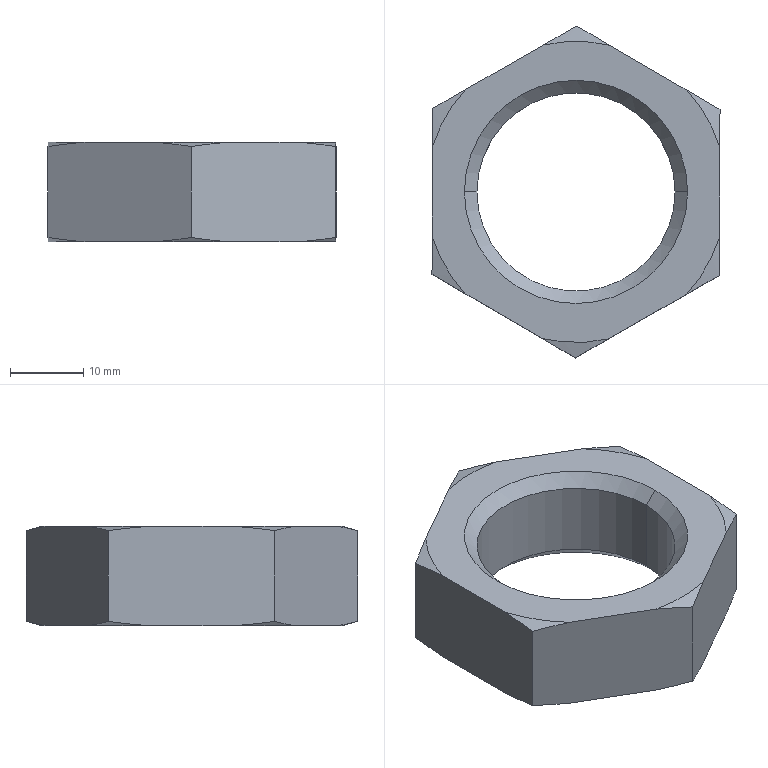Part | STEP file | GB/T6172.1-2000 hex thin nut grade A and B (M27) | 1 solid | 26 faces | box 39.233 x 45.2 x 13.5 mm | volume 9913 mm3 | cone 16 | plane 8 | cylinder 2 | commonest cylinder face diameters 27 x2
STEP:
#1=CARTESIAN_POINT('',(-13.5,0.,11.807));
#2=VERTEX_POINT('',#1);
#3=CARTESIAN_POINT('',(13.5,0.,11.807));
#4=VERTEX_POINT('',#3);
#5=CARTESIAN_POINT('',(0.,0.,11.807));
#6=DIRECTION('',(0.,0.,1.));
#7=DIRECTION('',(-1.,0.,0.));
#8=AXIS2_PLACEMENT_3D('',#5,#6,#7);
#9=CIRCLE('',#8,13.5);
#10=EDGE_CURVE('',#2,#4,#9,.T.);
#11=ORIENTED_EDGE('',*,*,#10,.F.);
#12=CARTESIAN_POINT('',(-15.193,0.,13.5));
#13=VERTEX_POINT('',#12);
#14=CARTESIAN_POINT('',(-13.5,0.,11.807));
#15=DIRECTION('',(-0.7071,0.,0.7071));
#16=VECTOR('',#15,1000.);
#17=LINE('',#14,#16);
#18=EDGE_CURVE('',#2,#13,#17,.T.);
#19=ORIENTED_EDGE('',*,*,#18,.T.);
#20=CARTESIAN_POINT('',(15.193,0.,13.5));
#21=VERTEX_POINT('',#20);
#22=CARTESIAN_POINT('',(0.,0.,13.5));
#23=DIRECTION('',(0.,0.,-1.));
#24=DIRECTION('',(-1.,0.,0.));
#25=AXIS2_PLACEMENT_3D('',#22,#23,#24);
#26=CIRCLE('',#25,15.193);
#27=EDGE_CURVE('',#21,#13,#26,.T.);
#28=ORIENTED_EDGE('',*,*,#27,.F.);
#29=CARTESIAN_POINT('',(13.5,0.,11.807));
#30=DIRECTION('',(0.7071,0.,0.7071));
#31=VECTOR('',#30,1000.);
#32=LINE('',#29,#31);
#33=EDGE_CURVE('',#4,#21,#32,.T.);
#34=ORIENTED_EDGE('',*,*,#33,.F.);
#35=EDGE_LOOP('',(#11,#19,#28,#34));
#36=FACE_OUTER_BOUND('',#35,.T.);
#37=CARTESIAN_POINT('',(0.,0.,11.807));
#38=DIRECTION('',(0.,0.,1.));
#39=DIRECTION('',(1.,0.,0.));
#40=AXIS2_PLACEMENT_3D('',#37,#38,#39);
#41=CONICAL_SURFACE('',#40,13.5,0.7854);
#42=ADVANCED_FACE('',(#36),#41,.F.);
#43=CARTESIAN_POINT('',(13.5,0.,1.693));
#44=VERTEX_POINT('',#43);
#45=CARTESIAN_POINT('',(-13.5,0.,1.693));
#46=VERTEX_POINT('',#45);
#47=CARTESIAN_POINT('',(0.,0.,1.693));
#48=DIRECTION('',(0.,0.,-1.));
#49=DIRECTION('',(-1.,0.,0.));
#50=AXIS2_PLACEMENT_3D('',#47,#48,#49);
#51=CIRCLE('',#50,13.5);
#52=EDGE_CURVE('',#44,#46,#51,.T.);
#53=ORIENTED_EDGE('',*,*,#52,.F.);
#54=CARTESIAN_POINT('',(15.193,0.,0.));
#55=VERTEX_POINT('',#54);
#56=CARTESIAN_POINT('',(15.193,0.,0.));
#57=DIRECTION('',(0.7071,0.,-0.7071));
#58=VECTOR('',#57,1000.);
#59=LINE('',#56,#58);
#60=EDGE_CURVE('',#44,#55,#59,.T.);
#61=ORIENTED_EDGE('',*,*,#60,.T.);
#62=CARTESIAN_POINT('',(-15.193,0.,0.));
#63=VERTEX_POINT('',#62);
#64=CARTESIAN_POINT('',(0.,0.,0.));
#65=DIRECTION('',(0.,0.,1.));
#66=DIRECTION('',(-1.,0.,0.));
#67=AXIS2_PLACEMENT_3D('',#64,#65,#66);
#68=CIRCLE('',#67,15.193);
#69=EDGE_CURVE('',#63,#55,#68,.T.);
#70=ORIENTED_EDGE('',*,*,#69,.F.);
#71=CARTESIAN_POINT('',(-15.193,0.,0.));
#72=DIRECTION('',(-0.7071,0.,-0.7071));
#73=VECTOR('',#72,1000.);
#74=LINE('',#71,#73);
#75=EDGE_CURVE('',#46,#63,#74,.T.);
#76=ORIENTED_EDGE('',*,*,#75,.F.);
#77=EDGE_LOOP('',(#53,#61,#70,#76));
#78=FACE_OUTER_BOUND('',#77,.T.);
#79=CARTESIAN_POINT('',(0.,0.,0.));
#80=DIRECTION('',(0.,0.,-1.));
#81=DIRECTION('',(-1.,0.,0.));
#82=AXIS2_PLACEMENT_3D('',#79,#80,#81);
#83=CONICAL_SURFACE('',#82,15.193,0.7854);
#84=ADVANCED_FACE('',(#78),#83,.F.);
#85=ORIENTED_EDGE('',*,*,#10,.T.);
#86=CARTESIAN_POINT('',(13.5,0.,13.5));
#87=DIRECTION('',(0.,0.,-1.));
#88=VECTOR('',#87,1000.);
#89=LINE('',#86,#88);
#90=EDGE_CURVE('',#4,#44,#89,.T.);
#91=ORIENTED_EDGE('',*,*,#90,.T.);
#92=ORIENTED_EDGE('',*,*,#52,.T.);
#93=CARTESIAN_POINT('',(-13.5,0.,13.5));
#94=DIRECTION('',(0.,0.,-1.));
#95=VECTOR('',#94,1000.);
#96=LINE('',#93,#95);
#97=EDGE_CURVE('',#2,#46,#96,.T.);
#98=ORIENTED_EDGE('',*,*,#97,.F.);
#99=EDGE_LOOP('',(#85,#91,#92,#98));
#100=FACE_OUTER_BOUND('',#99,.T.);
#101=CARTESIAN_POINT('',(0.,0.,13.5));
#102=DIRECTION('',(0.,0.,-1.));
#103=DIRECTION('',(-1.,0.,0.));
#104=AXIS2_PLACEMENT_3D('',#101,#102,#103);
#105=CYLINDRICAL_SURFACE('',#104,13.5);
#106=ADVANCED_FACE('',(#100),#105,.F.);
#107=CARTESIAN_POINT('',(19.616,11.223,12.937));
#108=VERTEX_POINT('',#107);
#109=CARTESIAN_POINT('',(15.121,13.842,13.5));
#110=VERTEX_POINT('',#109);
#111=CARTESIAN_POINT('',(19.616,11.223,12.937));
#112=CARTESIAN_POINT('',(18.122,12.093,13.169));
#113=CARTESIAN_POINT('',(16.624,12.966,13.361));
#114=CARTESIAN_POINT('',(15.121,13.842,13.5));
#115=B_SPLINE_CURVE_WITH_KNOTS('',3,(#111,#112,#113,#114),.UNSPECIFIED.,.F.,.F.,(4,4),(0.01855,0.02378),.UNSPECIFIED.);
#116=EDGE_CURVE('',#108,#110,#115,.T.);
#117=ORIENTED_EDGE('',*,*,#116,.F.);
#118=CARTESIAN_POINT('',(19.616,11.223,0.5627));
#119=VERTEX_POINT('',#118);
#120=CARTESIAN_POINT('',(19.616,11.223,13.5));
#121=DIRECTION('',(0.,0.,-1.));
#122=VECTOR('',#121,1000.);
#123=LINE('',#120,#122);
#124=EDGE_CURVE('',#108,#119,#123,.T.);
#125=ORIENTED_EDGE('',*,*,#124,.T.);
#126=CARTESIAN_POINT('',(15.121,13.842,0.));
#127=VERTEX_POINT('',#126);
#128=CARTESIAN_POINT('',(15.121,13.842,0.));
#129=CARTESIAN_POINT('',(16.625,12.966,0.1387));
#130=CARTESIAN_POINT('',(18.125,12.092,0.3314));
#131=CARTESIAN_POINT('',(19.616,11.223,0.5627));
#132=B_SPLINE_CURVE_WITH_KNOTS('',3,(#128,#129,#130,#131),.UNSPECIFIED.,.F.,.F.,(4,4),(0.0359,0.04105),.UNSPECIFIED.);
#133=EDGE_CURVE('',#127,#119,#132,.T.);
#134=ORIENTED_EDGE('',*,*,#133,.F.);
#135=CARTESIAN_POINT('',(4.584,19.981,0.));
#136=VERTEX_POINT('',#135);
#137=CARTESIAN_POINT('',(19.616,11.223,0.));
#138=DIRECTION('',(-0.8641,0.5034,0.));
#139=VECTOR('',#138,1000.);
#140=LINE('',#137,#139);
#141=EDGE_CURVE('',#127,#136,#140,.T.);
#142=ORIENTED_EDGE('',*,*,#141,.T.);
#143=CARTESIAN_POINT('',(0.0889,22.6,0.5627));
#144=VERTEX_POINT('',#143);
#145=CARTESIAN_POINT('',(0.0889,22.6,0.5627));
#146=CARTESIAN_POINT('',(1.583,21.729,0.331));
#147=CARTESIAN_POINT('',(3.081,20.857,0.1386));
#148=CARTESIAN_POINT('',(4.584,19.981,0.));
#149=B_SPLINE_CURVE_WITH_KNOTS('',3,(#145,#146,#147,#148),.UNSPECIFIED.,.F.,.F.,(4,4),(0.01855,0.02378),.UNSPECIFIED.);
#150=EDGE_CURVE('',#144,#136,#149,.T.);
#151=ORIENTED_EDGE('',*,*,#150,.F.);
#152=CARTESIAN_POINT('',(0.0889,22.6,12.937));
#153=VERTEX_POINT('',#152);
#154=CARTESIAN_POINT('',(0.0889,22.6,13.5));
#155=DIRECTION('',(0.,0.,-1.));
#156=VECTOR('',#155,1000.);
#157=LINE('',#154,#156);
#158=EDGE_CURVE('',#153,#144,#157,.T.);
#159=ORIENTED_EDGE('',*,*,#158,.F.);
#160=CARTESIAN_POINT('',(4.584,19.981,13.5));
#161=VERTEX_POINT('',#160);
#162=CARTESIAN_POINT('',(4.584,19.981,13.5));
#163=CARTESIAN_POINT('',(3.08,20.857,13.361));
#164=CARTESIAN_POINT('',(1.581,21.731,13.169));
#165=CARTESIAN_POINT('',(0.0889,22.6,12.937));
#166=B_SPLINE_CURVE_WITH_KNOTS('',3,(#162,#163,#164,#165),.UNSPECIFIED.,.F.,.F.,(4,4),(0.0359,0.04105),.UNSPECIFIED.);
#167=EDGE_CURVE('',#161,#153,#166,.T.);
#168=ORIENTED_EDGE('',*,*,#167,.F.);
#169=CARTESIAN_POINT('',(19.616,11.223,13.5));
#170=DIRECTION('',(-0.8641,0.5034,0.));
#171=VECTOR('',#170,1000.);
#172=LINE('',#169,#171);
#173=EDGE_CURVE('',#110,#161,#172,.T.);
#174=ORIENTED_EDGE('',*,*,#173,.F.);
#175=EDGE_LOOP('',(#117,#125,#134,#142,#151,#159,#168,#174));
#176=FACE_OUTER_BOUND('',#175,.T.);
#177=CARTESIAN_POINT('',(19.616,11.223,13.5));
#178=DIRECTION('',(-0.5034,-0.8641,0.));
#179=DIRECTION('',(0.8641,-0.5034,0.));
#180=AXIS2_PLACEMENT_3D('',#177,#178,#179);
#181=PLANE('',#180);
#182=ADVANCED_FACE('',(#176),#181,.F.);
#183=CARTESIAN_POINT('',(-4.427,20.016,13.5));
#184=VERTEX_POINT('',#183);
#185=CARTESIAN_POINT('',(0.0889,22.6,12.937));
#186=CARTESIAN_POINT('',(-1.412,21.741,13.169));
#187=CARTESIAN_POINT('',(-2.917,20.88,13.361));
#188=CARTESIAN_POINT('',(-4.427,20.016,13.5));
#189=B_SPLINE_CURVE_WITH_KNOTS('',3,(#185,#186,#187,#188),.UNSPECIFIED.,.F.,.F.,(4,4),(0.01846,0.0237),.UNSPECIFIED.);
#190=EDGE_CURVE('',#153,#184,#189,.T.);
#191=ORIENTED_EDGE('',*,*,#190,.F.);
#192=ORIENTED_EDGE('',*,*,#158,.T.);
#193=CARTESIAN_POINT('',(-4.427,20.016,0.));
#194=VERTEX_POINT('',#193);
#195=CARTESIAN_POINT('',(-4.427,20.016,0.));
#196=CARTESIAN_POINT('',(-2.916,20.881,0.1387));
#197=CARTESIAN_POINT('',(-1.41,21.742,0.3314));
#198=CARTESIAN_POINT('',(0.0889,22.6,0.5627));
#199=B_SPLINE_CURVE_WITH_KNOTS('',3,(#195,#196,#197,#198),.UNSPECIFIED.,.F.,.F.,(4,4),(0.03582,0.04096),.UNSPECIFIED.);
#200=EDGE_CURVE('',#194,#144,#199,.T.);
#201=ORIENTED_EDGE('',*,*,#200,.F.);
#202=CARTESIAN_POINT('',(-15.012,13.96,0.));
#203=VERTEX_POINT('',#202);
#204=CARTESIAN_POINT('',(0.0889,22.6,0.));
#205=DIRECTION('',(-0.868,-0.4966,0.));
#206=VECTOR('',#205,1000.);
#207=LINE('',#204,#206);
#208=EDGE_CURVE('',#194,#203,#207,.T.);
#209=ORIENTED_EDGE('',*,*,#208,.T.);
#210=CARTESIAN_POINT('',(-19.528,11.377,0.5627));
#211=VERTEX_POINT('',#210);
#212=CARTESIAN_POINT('',(-19.528,11.377,0.5627));
#213=CARTESIAN_POINT('',(-18.027,12.236,0.331));
#214=CARTESIAN_POINT('',(-16.522,13.097,0.1386));
#215=CARTESIAN_POINT('',(-15.012,13.96,0.));
#216=B_SPLINE_CURVE_WITH_KNOTS('',3,(#212,#213,#214,#215),.UNSPECIFIED.,.F.,.F.,(4,4),(0.01846,0.0237),.UNSPECIFIED.);
#217=EDGE_CURVE('',#211,#203,#216,.T.);
#218=ORIENTED_EDGE('',*,*,#217,.F.);
#219=CARTESIAN_POINT('',(-19.528,11.377,12.937));
#220=VERTEX_POINT('',#219);
#221=CARTESIAN_POINT('',(-19.528,11.377,13.5));
#222=DIRECTION('',(0.,0.,-1.));
#223=VECTOR('',#222,1000.);
#224=LINE('',#221,#223);
#225=EDGE_CURVE('',#220,#211,#224,.T.);
#226=ORIENTED_EDGE('',*,*,#225,.F.);
#227=CARTESIAN_POINT('',(-15.012,13.96,13.5));
#228=VERTEX_POINT('',#227);
#229=CARTESIAN_POINT('',(-15.012,13.96,13.5));
#230=CARTESIAN_POINT('',(-16.522,13.096,13.361));
#231=CARTESIAN_POINT('',(-18.029,12.234,13.169));
#232=CARTESIAN_POINT('',(-19.528,11.377,12.937));
#233=B_SPLINE_CURVE_WITH_KNOTS('',3,(#229,#230,#231,#232),.UNSPECIFIED.,.F.,.F.,(4,4),(0.03582,0.04096),.UNSPECIFIED.);
#234=EDGE_CURVE('',#228,#220,#233,.T.);
#235=ORIENTED_EDGE('',*,*,#234,.F.);
#236=CARTESIAN_POINT('',(0.0889,22.6,13.5));
#237=DIRECTION('',(-0.868,-0.4966,0.));
#238=VECTOR('',#237,1000.);
#239=LINE('',#236,#238);
#240=EDGE_CURVE('',#184,#228,#239,.T.);
#241=ORIENTED_EDGE('',*,*,#240,.F.);
#242=EDGE_LOOP('',(#191,#192,#201,#209,#218,#226,#235,#241));
#243=FACE_OUTER_BOUND('',#242,.T.);
#244=CARTESIAN_POINT('',(0.0889,22.6,13.5));
#245=DIRECTION('',(0.4966,-0.868,0.));
#246=DIRECTION('',(0.868,0.4966,0.));
#247=AXIS2_PLACEMENT_3D('',#244,#245,#246);
#248=PLANE('',#247);
#249=ADVANCED_FACE('',(#243),#248,.F.);
#250=CARTESIAN_POINT('',(-19.548,6.174,13.5));
#251=VERTEX_POINT('',#250);
#252=CARTESIAN_POINT('',(-19.528,11.377,12.937));
#253=CARTESIAN_POINT('',(-19.534,9.647,13.169));
#254=CARTESIAN_POINT('',(-19.541,7.913,13.361));
#255=CARTESIAN_POINT('',(-19.548,6.174,13.5));
#256=B_SPLINE_CURVE_WITH_KNOTS('',3,(#252,#253,#254,#255),.UNSPECIFIED.,.F.,.F.,(4,4),(0.016,0.02124),.UNSPECIFIED.);
#257=EDGE_CURVE('',#220,#251,#256,.T.);
#258=ORIENTED_EDGE('',*,*,#257,.F.);
#259=ORIENTED_EDGE('',*,*,#225,.T.);
#260=CARTESIAN_POINT('',(-19.548,6.174,0.));
#261=VERTEX_POINT('',#260);
#262=CARTESIAN_POINT('',(-19.548,6.174,0.));
#263=CARTESIAN_POINT('',(-19.545,7.043,0.06926));
#264=CARTESIAN_POINT('',(-19.541,7.914,0.1522));
#265=CARTESIAN_POINT('',(-19.534,9.648,0.341));
#266=CARTESIAN_POINT('',(-19.531,10.513,0.447));
#267=CARTESIAN_POINT('',(-19.528,11.377,0.5627));
#268=B_SPLINE_CURVE_WITH_KNOTS('',3,(#262,#263,#264,#265,#266,#267),.UNSPECIFIED.,.F.,.F.,(4,2,4),(0.03337,0.03595,0.03852),.UNSPECIFIED.);
#269=EDGE_CURVE('',#261,#211,#268,.T.);
#270=ORIENTED_EDGE('',*,*,#269,.F.);
#271=CARTESIAN_POINT('',(-19.596,-6.021,0.));
#272=VERTEX_POINT('',#271);
#273=CARTESIAN_POINT('',(-19.528,11.377,0.));
#274=DIRECTION('',(-0.003934,-1.,0.));
#275=VECTOR('',#274,1000.);
#276=LINE('',#273,#275);
#277=EDGE_CURVE('',#261,#272,#276,.T.);
#278=ORIENTED_EDGE('',*,*,#277,.T.);
#279=CARTESIAN_POINT('',(-19.616,-11.223,0.5627));
#280=VERTEX_POINT('',#279);
#281=CARTESIAN_POINT('',(-19.616,-11.223,0.5627));
#282=CARTESIAN_POINT('',(-19.61,-9.493,0.3309));
#283=CARTESIAN_POINT('',(-19.603,-7.76,0.1386));
#284=CARTESIAN_POINT('',(-19.596,-6.021,0.));
#285=B_SPLINE_CURVE_WITH_KNOTS('',3,(#281,#282,#283,#284),.UNSPECIFIED.,.F.,.F.,(4,4),(0.016,0.02124),.UNSPECIFIED.);
#286=EDGE_CURVE('',#280,#272,#285,.T.);
#287=ORIENTED_EDGE('',*,*,#286,.F.);
#288=CARTESIAN_POINT('',(-19.616,-11.223,12.937));
#289=VERTEX_POINT('',#288);
#290=CARTESIAN_POINT('',(-19.616,-11.223,13.5));
#291=DIRECTION('',(0.,0.,-1.));
#292=VECTOR('',#291,1000.);
#293=LINE('',#290,#292);
#294=EDGE_CURVE('',#289,#280,#293,.T.);
#295=ORIENTED_EDGE('',*,*,#294,.F.);
#296=CARTESIAN_POINT('',(-19.596,-6.021,13.5));
#297=VERTEX_POINT('',#296);
#298=CARTESIAN_POINT('',(-19.596,-6.021,13.5));
#299=CARTESIAN_POINT('',(-19.599,-6.89,13.431));
#300=CARTESIAN_POINT('',(-19.603,-7.76,13.348));
#301=CARTESIAN_POINT('',(-19.61,-9.494,13.159));
#302=CARTESIAN_POINT('',(-19.613,-10.359,13.053));
#303=CARTESIAN_POINT('',(-19.616,-11.223,12.937));
#304=B_SPLINE_CURVE_WITH_KNOTS('',3,(#298,#299,#300,#301,#302,#303),.UNSPECIFIED.,.F.,.F.,(4,2,4),(0.03337,0.03595,0.03852),.UNSPECIFIED.);
#305=EDGE_CURVE('',#297,#289,#304,.T.);
#306=ORIENTED_EDGE('',*,*,#305,.F.);
#307=CARTESIAN_POINT('',(-19.528,11.377,13.5));
#308=DIRECTION('',(-0.003934,-1.,0.));
#309=VECTOR('',#308,1000.);
#310=LINE('',#307,#309);
#311=EDGE_CURVE('',#251,#297,#310,.T.);
#312=ORIENTED_EDGE('',*,*,#311,.F.);
#313=EDGE_LOOP('',(#258,#259,#270,#278,#287,#295,#306,#312));
#314=FACE_OUTER_BOUND('',#313,.T.);
#315=CARTESIAN_POINT('',(-19.528,11.377,13.5));
#316=DIRECTION('',(1.,-0.003934,0.));
#317=DIRECTION('',(0.003934,1.,0.));
#318=AXIS2_PLACEMENT_3D('',#315,#316,#317);
#319=PLANE('',#318);
#320=ADVANCED_FACE('',(#314),#319,.F.);
#321=CARTESIAN_POINT('',(-15.121,-13.842,13.5));
#322=VERTEX_POINT('',#321);
#323=CARTESIAN_POINT('',(-19.616,-11.223,12.937));
#324=CARTESIAN_POINT('',(-18.122,-12.093,13.169));
#325=CARTESIAN_POINT('',(-16.624,-12.966,13.361));
#326=CARTESIAN_POINT('',(-15.121,-13.842,13.5));
#327=B_SPLINE_CURVE_WITH_KNOTS('',3,(#323,#324,#325,#326),.UNSPECIFIED.,.F.,.F.,(4,4),(0.01855,0.02378),.UNSPECIFIED.);
#328=EDGE_CURVE('',#289,#322,#327,.T.);
#329=ORIENTED_EDGE('',*,*,#328,.F.);
#330=ORIENTED_EDGE('',*,*,#294,.T.);
#331=CARTESIAN_POINT('',(-15.121,-13.842,0.));
#332=VERTEX_POINT('',#331);
#333=CARTESIAN_POINT('',(-15.121,-13.842,0.));
#334=CARTESIAN_POINT('',(-16.625,-12.966,0.1387));
#335=CARTESIAN_POINT('',(-18.125,-12.092,0.3314));
#336=CARTESIAN_POINT('',(-19.616,-11.223,0.5627));
#337=B_SPLINE_CURVE_WITH_KNOTS('',3,(#333,#334,#335,#336),.UNSPECIFIED.,.F.,.F.,(4,4),(0.0359,0.04105),.UNSPECIFIED.);
#338=EDGE_CURVE('',#332,#280,#337,.T.);
#339=ORIENTED_EDGE('',*,*,#338,.F.);
#340=CARTESIAN_POINT('',(-4.584,-19.981,0.));
#341=VERTEX_POINT('',#340);
#342=CARTESIAN_POINT('',(-19.616,-11.223,0.));
#343=DIRECTION('',(0.8641,-0.5034,0.));
#344=VECTOR('',#343,1000.);
#345=LINE('',#342,#344);
#346=EDGE_CURVE('',#332,#341,#345,.T.);
#347=ORIENTED_EDGE('',*,*,#346,.T.);
#348=CARTESIAN_POINT('',(-0.0889,-22.6,0.5627));
#349=VERTEX_POINT('',#348);
#350=CARTESIAN_POINT('',(-0.0889,-22.6,0.5627));
#351=CARTESIAN_POINT('',(-1.583,-21.729,0.331));
#352=CARTESIAN_POINT('',(-3.081,-20.857,0.1386));
#353=CARTESIAN_POINT('',(-4.584,-19.981,0.));
#354=B_SPLINE_CURVE_WITH_KNOTS('',3,(#350,#351,#352,#353),.UNSPECIFIED.,.F.,.F.,(4,4),(0.01855,0.02378),.UNSPECIFIED.);
#355=EDGE_CURVE('',#349,#341,#354,.T.);
#356=ORIENTED_EDGE('',*,*,#355,.F.);
#357=CARTESIAN_POINT('',(-0.0889,-22.6,12.937));
#358=VERTEX_POINT('',#357);
#359=CARTESIAN_POINT('',(-0.0889,-22.6,13.5));
#360=DIRECTION('',(0.,0.,-1.));
#361=VECTOR('',#360,1000.);
#362=LINE('',#359,#361);
#363=EDGE_CURVE('',#358,#349,#362,.T.);
#364=ORIENTED_EDGE('',*,*,#363,.F.);
#365=CARTESIAN_POINT('',(-4.584,-19.981,13.5));
#366=VERTEX_POINT('',#365);
#367=CARTESIAN_POINT('',(-4.584,-19.981,13.5));
#368=CARTESIAN_POINT('',(-3.08,-20.857,13.361));
#369=CARTESIAN_POINT('',(-1.581,-21.731,13.169));
#370=CARTESIAN_POINT('',(-0.0889,-22.6,12.937));
#371=B_SPLINE_CURVE_WITH_KNOTS('',3,(#367,#368,#369,#370),.UNSPECIFIED.,.F.,.F.,(4,4),(0.0359,0.04105),.UNSPECIFIED.);
#372=EDGE_CURVE('',#366,#358,#371,.T.);
#373=ORIENTED_EDGE('',*,*,#372,.F.);
#374=CARTESIAN_POINT('',(-19.616,-11.223,13.5));
#375=DIRECTION('',(0.8641,-0.5034,0.));
#376=VECTOR('',#375,1000.);
#377=LINE('',#374,#376);
#378=EDGE_CURVE('',#322,#366,#377,.T.);
#379=ORIENTED_EDGE('',*,*,#378,.F.);
#380=EDGE_LOOP('',(#329,#330,#339,#347,#356,#364,#373,#379));
#381=FACE_OUTER_BOUND('',#380,.T.);
#382=CARTESIAN_POINT('',(-19.616,-11.223,13.5));
#383=DIRECTION('',(0.5034,0.8641,0.));
#384=DIRECTION('',(-0.8641,0.5034,0.));
#385=AXIS2_PLACEMENT_3D('',#382,#383,#384);
#386=PLANE('',#385);
#387=ADVANCED_FACE('',(#381),#386,.F.);
#388=CARTESIAN_POINT('',(4.427,-20.016,13.5));
#389=VERTEX_POINT('',#388);
#390=CARTESIAN_POINT('',(-0.0889,-22.6,12.937));
#391=CARTESIAN_POINT('',(1.412,-21.741,13.169));
#392=CARTESIAN_POINT('',(2.917,-20.88,13.361));
#393=CARTESIAN_POINT('',(4.427,-20.016,13.5));
#394=B_SPLINE_CURVE_WITH_KNOTS('',3,(#390,#391,#392,#393),.UNSPECIFIED.,.F.,.F.,(4,4),(0.01846,0.0237),.UNSPECIFIED.);
#395=EDGE_CURVE('',#358,#389,#394,.T.);
#396=ORIENTED_EDGE('',*,*,#395,.F.);
#397=ORIENTED_EDGE('',*,*,#363,.T.);
#398=CARTESIAN_POINT('',(4.427,-20.016,0.));
#399=VERTEX_POINT('',#398);
#400=CARTESIAN_POINT('',(4.427,-20.016,0.));
#401=CARTESIAN_POINT('',(2.916,-20.881,0.1387));
#402=CARTESIAN_POINT('',(1.41,-21.742,0.3314));
#403=CARTESIAN_POINT('',(-0.0889,-22.6,0.5627));
#404=B_SPLINE_CURVE_WITH_KNOTS('',3,(#400,#401,#402,#403),.UNSPECIFIED.,.F.,.F.,(4,4),(0.03582,0.04096),.UNSPECIFIED.);
#405=EDGE_CURVE('',#399,#349,#404,.T.);
#406=ORIENTED_EDGE('',*,*,#405,.F.);
#407=CARTESIAN_POINT('',(15.012,-13.96,0.));
#408=VERTEX_POINT('',#407);
#409=CARTESIAN_POINT('',(-0.0889,-22.6,0.));
#410=DIRECTION('',(0.868,0.4966,0.));
#411=VECTOR('',#410,1000.);
#412=LINE('',#409,#411);
#413=EDGE_CURVE('',#399,#408,#412,.T.);
#414=ORIENTED_EDGE('',*,*,#413,.T.);
#415=CARTESIAN_POINT('',(19.528,-11.377,0.5627));
#416=VERTEX_POINT('',#415);
#417=CARTESIAN_POINT('',(19.528,-11.377,0.5627));
#418=CARTESIAN_POINT('',(18.027,-12.236,0.331));
#419=CARTESIAN_POINT('',(16.522,-13.097,0.1386));
#420=CARTESIAN_POINT('',(15.012,-13.96,0.));
#421=B_SPLINE_CURVE_WITH_KNOTS('',3,(#417,#418,#419,#420),.UNSPECIFIED.,.F.,.F.,(4,4),(0.01846,0.0237),.UNSPECIFIED.);
#422=EDGE_CURVE('',#416,#408,#421,.T.);
#423=ORIENTED_EDGE('',*,*,#422,.F.);
#424=CARTESIAN_POINT('',(19.528,-11.377,12.937));
#425=VERTEX_POINT('',#424);
#426=CARTESIAN_POINT('',(19.528,-11.377,13.5));
#427=DIRECTION('',(0.,0.,-1.));
#428=VECTOR('',#427,1000.);
#429=LINE('',#426,#428);
#430=EDGE_CURVE('',#425,#416,#429,.T.);
#431=ORIENTED_EDGE('',*,*,#430,.F.);
#432=CARTESIAN_POINT('',(15.012,-13.96,13.5));
#433=VERTEX_POINT('',#432);
#434=CARTESIAN_POINT('',(15.012,-13.96,13.5));
#435=CARTESIAN_POINT('',(16.522,-13.096,13.361));
#436=CARTESIAN_POINT('',(18.029,-12.234,13.169));
#437=CARTESIAN_POINT('',(19.528,-11.377,12.937));
#438=B_SPLINE_CURVE_WITH_KNOTS('',3,(#434,#435,#436,#437),.UNSPECIFIED.,.F.,.F.,(4,4),(0.03582,0.04096),.UNSPECIFIED.);
#439=EDGE_CURVE('',#433,#425,#438,.T.);
#440=ORIENTED_EDGE('',*,*,#439,.F.);
#441=CARTESIAN_POINT('',(-0.0889,-22.6,13.5));
#442=DIRECTION('',(0.868,0.4966,0.));
#443=VECTOR('',#442,1000.);
#444=LINE('',#441,#443);
#445=EDGE_CURVE('',#389,#433,#444,.T.);
#446=ORIENTED_EDGE('',*,*,#445,.F.);
#447=EDGE_LOOP('',(#396,#397,#406,#414,#423,#431,#440,#446));
#448=FACE_OUTER_BOUND('',#447,.T.);
#449=CARTESIAN_POINT('',(-0.0889,-22.6,13.5));
#450=DIRECTION('',(-0.4966,0.868,0.));
#451=DIRECTION('',(-0.868,-0.4966,0.));
#452=AXIS2_PLACEMENT_3D('',#449,#450,#451);
#453=PLANE('',#452);
#454=ADVANCED_FACE('',(#448),#453,.F.);
#455=CARTESIAN_POINT('',(19.548,-6.174,13.5));
#456=VERTEX_POINT('',#455);
#457=CARTESIAN_POINT('',(19.528,-11.377,12.937));
#458=CARTESIAN_POINT('',(19.534,-9.647,13.169));
#459=CARTESIAN_POINT('',(19.541,-7.913,13.361));
#460=CARTESIAN_POINT('',(19.548,-6.174,13.5));
#461=B_SPLINE_CURVE_WITH_KNOTS('',3,(#457,#458,#459,#460),.UNSPECIFIED.,.F.,.F.,(4,4),(0.016,0.02124),.UNSPECIFIED.);
#462=EDGE_CURVE('',#425,#456,#461,.T.);
#463=ORIENTED_EDGE('',*,*,#462,.F.);
#464=ORIENTED_EDGE('',*,*,#430,.T.);
#465=CARTESIAN_POINT('',(19.548,-6.174,0.));
#466=VERTEX_POINT('',#465);
#467=CARTESIAN_POINT('',(19.548,-6.174,0.));
#468=CARTESIAN_POINT('',(19.545,-7.043,0.06926));
#469=CARTESIAN_POINT('',(19.541,-7.914,0.1522));
#470=CARTESIAN_POINT('',(19.534,-9.648,0.341));
#471=CARTESIAN_POINT('',(19.531,-10.513,0.447));
#472=CARTESIAN_POINT('',(19.528,-11.377,0.5627));
#473=B_SPLINE_CURVE_WITH_KNOTS('',3,(#467,#468,#469,#470,#471,#472),.UNSPECIFIED.,.F.,.F.,(4,2,4),(0.03337,0.03595,0.03852),.UNSPECIFIED.);
#474=EDGE_CURVE('',#466,#416,#473,.T.);
#475=ORIENTED_EDGE('',*,*,#474,.F.);
#476=CARTESIAN_POINT('',(19.596,6.021,0.));
#477=VERTEX_POINT('',#476);
#478=CARTESIAN_POINT('',(19.528,-11.377,0.));
#479=DIRECTION('',(0.003934,1.,0.));
#480=VECTOR('',#479,1000.);
#481=LINE('',#478,#480);
#482=EDGE_CURVE('',#466,#477,#481,.T.);
#483=ORIENTED_EDGE('',*,*,#482,.T.);
#484=CARTESIAN_POINT('',(19.616,11.223,0.5627));
#485=CARTESIAN_POINT('',(19.61,9.493,0.3309));
#486=CARTESIAN_POINT('',(19.603,7.76,0.1386));
#487=CARTESIAN_POINT('',(19.596,6.021,0.));
#488=B_SPLINE_CURVE_WITH_KNOTS('',3,(#484,#485,#486,#487),.UNSPECIFIED.,.F.,.F.,(4,4),(0.016,0.02124),.UNSPECIFIED.);
#489=EDGE_CURVE('',#119,#477,#488,.T.);
#490=ORIENTED_EDGE('',*,*,#489,.F.);
#491=ORIENTED_EDGE('',*,*,#124,.F.);
#492=CARTESIAN_POINT('',(19.596,6.021,13.5));
#493=VERTEX_POINT('',#492);
#494=CARTESIAN_POINT('',(19.596,6.021,13.5));
#495=CARTESIAN_POINT('',(19.599,6.89,13.431));
#496=CARTESIAN_POINT('',(19.603,7.76,13.348));
#497=CARTESIAN_POINT('',(19.61,9.494,13.159));
#498=CARTESIAN_POINT('',(19.613,10.359,13.053));
#499=CARTESIAN_POINT('',(19.616,11.223,12.937));
#500=B_SPLINE_CURVE_WITH_KNOTS('',3,(#494,#495,#496,#497,#498,#499),.UNSPECIFIED.,.F.,.F.,(4,2,4),(0.03337,0.03595,0.03852),.UNSPECIFIED.);
#501=EDGE_CURVE('',#493,#108,#500,.T.);
#502=ORIENTED_EDGE('',*,*,#501,.F.);
#503=CARTESIAN_POINT('',(19.528,-11.377,13.5));
#504=DIRECTION('',(0.003934,1.,0.));
#505=VECTOR('',#504,1000.);
#506=LINE('',#503,#505);
#507=EDGE_CURVE('',#456,#493,#506,.T.);
#508=ORIENTED_EDGE('',*,*,#507,.F.);
#509=EDGE_LOOP('',(#463,#464,#475,#483,#490,#491,#502,#508));
#510=FACE_OUTER_BOUND('',#509,.T.);
#511=CARTESIAN_POINT('',(19.528,-11.377,13.5));
#512=DIRECTION('',(-1.,0.003934,0.));
#513=DIRECTION('',(-0.003934,-1.,0.));
#514=AXIS2_PLACEMENT_3D('',#511,#512,#513);
#515=PLANE('',#514);
#516=ADVANCED_FACE('',(#510),#515,.F.);
#517=ORIENTED_EDGE('',*,*,#27,.T.);
#518=CARTESIAN_POINT('',(0.,0.,13.5));
#519=DIRECTION('',(0.,0.,-1.));
#520=DIRECTION('',(-1.,0.,0.));
#521=AXIS2_PLACEMENT_3D('',#518,#519,#520);
#522=CIRCLE('',#521,15.193);
#523=EDGE_CURVE('',#13,#21,#522,.T.);
#524=ORIENTED_EDGE('',*,*,#523,.T.);
#525=EDGE_LOOP('',(#517,#524));
#526=FACE_BOUND('',#525,.T.);
#527=CARTESIAN_POINT('',(0.,0.,13.5));
#528=DIRECTION('',(0.,0.,-1.));
#529=DIRECTION('',(-1.,0.,0.));
#530=AXIS2_PLACEMENT_3D('',#527,#528,#529);
#531=CIRCLE('',#530,20.5);
#532=EDGE_CURVE('',#251,#228,#531,.T.);
#533=ORIENTED_EDGE('',*,*,#532,.F.);
#534=ORIENTED_EDGE('',*,*,#311,.T.);
#535=CARTESIAN_POINT('',(0.,0.,13.5));
#536=DIRECTION('',(0.,0.,-1.));
#537=DIRECTION('',(-1.,0.,0.));
#538=AXIS2_PLACEMENT_3D('',#535,#536,#537);
#539=CIRCLE('',#538,20.5);
#540=EDGE_CURVE('',#322,#297,#539,.T.);
#541=ORIENTED_EDGE('',*,*,#540,.F.);
#542=ORIENTED_EDGE('',*,*,#378,.T.);
#543=CARTESIAN_POINT('',(0.,0.,13.5));
#544=DIRECTION('',(0.,0.,-1.));
#545=DIRECTION('',(-1.,0.,0.));
#546=AXIS2_PLACEMENT_3D('',#543,#544,#545);
#547=CIRCLE('',#546,20.5);
#548=EDGE_CURVE('',#389,#366,#547,.T.);
#549=ORIENTED_EDGE('',*,*,#548,.F.);
#550=ORIENTED_EDGE('',*,*,#445,.T.);
#551=CARTESIAN_POINT('',(0.,0.,13.5));
#552=DIRECTION('',(0.,0.,-1.));
#553=DIRECTION('',(-1.,0.,0.));
#554=AXIS2_PLACEMENT_3D('',#551,#552,#553);
#555=CIRCLE('',#554,20.5);
#556=EDGE_CURVE('',#456,#433,#555,.T.);
#557=ORIENTED_EDGE('',*,*,#556,.F.);
#558=ORIENTED_EDGE('',*,*,#507,.T.);
#559=CARTESIAN_POINT('',(0.,0.,13.5));
#560=DIRECTION('',(0.,0.,1.));
#561=DIRECTION('',(1.,0.,0.));
#562=AXIS2_PLACEMENT_3D('',#559,#560,#561);
#563=CIRCLE('',#562,20.5);
#564=EDGE_CURVE('',#493,#110,#563,.T.);
#565=ORIENTED_EDGE('',*,*,#564,.T.);
#566=ORIENTED_EDGE('',*,*,#173,.T.);
#567=CARTESIAN_POINT('',(0.,0.,13.5));
#568=DIRECTION('',(0.,0.,-1.));
#569=DIRECTION('',(-1.,0.,0.));
#570=AXIS2_PLACEMENT_3D('',#567,#568,#569);
#571=CIRCLE('',#570,20.5);
#572=EDGE_CURVE('',#184,#161,#571,.T.);
#573=ORIENTED_EDGE('',*,*,#572,.F.);
#574=ORIENTED_EDGE('',*,*,#240,.T.);
#575=EDGE_LOOP('',(#533,#534,#541,#542,#549,#550,#557,#558,#565,#566,#573,#574));
#576=FACE_OUTER_BOUND('',#575,.T.);
#577=CARTESIAN_POINT('',(19.616,11.223,13.5));
#578=DIRECTION('',(0.,0.,-1.));
#579=DIRECTION('',(-1.,0.,0.));
#580=AXIS2_PLACEMENT_3D('',#577,#578,#579);
#581=PLANE('',#580);
#582=ADVANCED_FACE('',(#526,#576),#581,.F.);
#583=ORIENTED_EDGE('',*,*,#69,.T.);
#584=CARTESIAN_POINT('',(0.,0.,0.));
#585=DIRECTION('',(0.,0.,1.));
#586=DIRECTION('',(-1.,0.,0.));
#587=AXIS2_PLACEMENT_3D('',#584,#585,#586);
#588=CIRCLE('',#587,15.193);
#589=EDGE_CURVE('',#55,#63,#588,.T.);
#590=ORIENTED_EDGE('',*,*,#589,.T.);
#591=EDGE_LOOP('',(#583,#590));
#592=FACE_BOUND('',#591,.T.);
#593=ORIENTED_EDGE('',*,*,#277,.F.);
#594=CARTESIAN_POINT('',(0.,0.,0.));
#595=DIRECTION('',(0.,0.,-1.));
#596=DIRECTION('',(-1.,0.,0.));
#597=AXIS2_PLACEMENT_3D('',#594,#595,#596);
#598=CIRCLE('',#597,20.5);
#599=EDGE_CURVE('',#261,#203,#598,.T.);
#600=ORIENTED_EDGE('',*,*,#599,.T.);
#601=ORIENTED_EDGE('',*,*,#208,.F.);
#602=CARTESIAN_POINT('',(0.,0.,0.));
#603=DIRECTION('',(0.,0.,-1.));
#604=DIRECTION('',(-1.,0.,0.));
#605=AXIS2_PLACEMENT_3D('',#602,#603,#604);
#606=CIRCLE('',#605,20.5);
#607=EDGE_CURVE('',#194,#136,#606,.T.);
#608=ORIENTED_EDGE('',*,*,#607,.T.);
#609=ORIENTED_EDGE('',*,*,#141,.F.);
#610=CARTESIAN_POINT('',(0.,0.,0.));
#611=DIRECTION('',(0.,0.,-1.));
#612=DIRECTION('',(-1.,0.,0.));
#613=AXIS2_PLACEMENT_3D('',#610,#611,#612);
#614=CIRCLE('',#613,20.5);
#615=EDGE_CURVE('',#127,#477,#614,.T.);
#616=ORIENTED_EDGE('',*,*,#615,.T.);
#617=ORIENTED_EDGE('',*,*,#482,.F.);
#618=CARTESIAN_POINT('',(0.,0.,0.));
#619=DIRECTION('',(0.,0.,-1.));
#620=DIRECTION('',(-1.,0.,0.));
#621=AXIS2_PLACEMENT_3D('',#618,#619,#620);
#622=CIRCLE('',#621,20.5);
#623=EDGE_CURVE('',#466,#408,#622,.T.);
#624=ORIENTED_EDGE('',*,*,#623,.T.);
#625=ORIENTED_EDGE('',*,*,#413,.F.);
#626=CARTESIAN_POINT('',(0.,0.,0.));
#627=DIRECTION('',(0.,0.,-1.));
#628=DIRECTION('',(-1.,0.,0.));
#629=AXIS2_PLACEMENT_3D('',#626,#627,#628);
#630=CIRCLE('',#629,20.5);
#631=EDGE_CURVE('',#399,#341,#630,.T.);
#632=ORIENTED_EDGE('',*,*,#631,.T.);
#633=ORIENTED_EDGE('',*,*,#346,.F.);
#634=CARTESIAN_POINT('',(0.,0.,0.));
#635=DIRECTION('',(0.,0.,-1.));
#636=DIRECTION('',(-1.,0.,0.));
#637=AXIS2_PLACEMENT_3D('',#634,#635,#636);
#638=CIRCLE('',#637,20.5);
#639=EDGE_CURVE('',#332,#272,#638,.T.);
#640=ORIENTED_EDGE('',*,*,#639,.T.);
#641=EDGE_LOOP('',(#593,#600,#601,#608,#609,#616,#617,#624,#625,#632,#633,#640));
#642=FACE_OUTER_BOUND('',#641,.T.);
#643=CARTESIAN_POINT('',(19.616,11.223,0.));
#644=DIRECTION('',(0.,0.,-1.));
#645=DIRECTION('',(-1.,0.,0.));
#646=AXIS2_PLACEMENT_3D('',#643,#644,#645);
#647=PLANE('',#646);
#648=ADVANCED_FACE('',(#592,#642),#647,.T.);
#649=ORIENTED_EDGE('',*,*,#90,.F.);
#650=CARTESIAN_POINT('',(0.,0.,11.807));
#651=DIRECTION('',(0.,0.,1.));
#652=DIRECTION('',(-1.,0.,0.));
#653=AXIS2_PLACEMENT_3D('',#650,#651,#652);
#654=CIRCLE('',#653,13.5);
#655=EDGE_CURVE('',#4,#2,#654,.T.);
#656=ORIENTED_EDGE('',*,*,#655,.T.);
#657=ORIENTED_EDGE('',*,*,#97,.T.);
#658=CARTESIAN_POINT('',(0.,0.,1.693));
#659=DIRECTION('',(0.,0.,-1.));
#660=DIRECTION('',(-1.,0.,0.));
#661=AXIS2_PLACEMENT_3D('',#658,#659,#660);
#662=CIRCLE('',#661,13.5);
#663=EDGE_CURVE('',#46,#44,#662,.T.);
#664=ORIENTED_EDGE('',*,*,#663,.T.);
#665=EDGE_LOOP('',(#649,#656,#657,#664));
#666=FACE_OUTER_BOUND('',#665,.T.);
#667=CARTESIAN_POINT('',(0.,0.,13.5));
#668=DIRECTION('',(0.,0.,-1.));
#669=DIRECTION('',(-1.,0.,0.));
#670=AXIS2_PLACEMENT_3D('',#667,#668,#669);
#671=CYLINDRICAL_SURFACE('',#670,13.5);
#672=ADVANCED_FACE('',(#666),#671,.F.);
#673=ORIENTED_EDGE('',*,*,#422,.T.);
#674=ORIENTED_EDGE('',*,*,#623,.F.);
#675=ORIENTED_EDGE('',*,*,#474,.T.);
#676=EDGE_LOOP('',(#673,#674,#675));
#677=FACE_OUTER_BOUND('',#676,.T.);
#678=CARTESIAN_POINT('',(0.,0.,0.));
#679=DIRECTION('',(0.,0.,1.));
#680=DIRECTION('',(-1.,0.,0.));
#681=AXIS2_PLACEMENT_3D('',#678,#679,#680);
#682=CONICAL_SURFACE('',#681,20.5,1.309);
#683=ADVANCED_FACE('',(#677),#682,.T.);
#684=ORIENTED_EDGE('',*,*,#133,.T.);
#685=ORIENTED_EDGE('',*,*,#489,.T.);
#686=ORIENTED_EDGE('',*,*,#615,.F.);
#687=EDGE_LOOP('',(#684,#685,#686));
#688=FACE_OUTER_BOUND('',#687,.T.);
#689=CARTESIAN_POINT('',(0.,0.,0.));
#690=DIRECTION('',(0.,0.,1.));
#691=DIRECTION('',(-1.,0.,0.));
#692=AXIS2_PLACEMENT_3D('',#689,#690,#691);
#693=CONICAL_SURFACE('',#692,20.5,1.309);
#694=ADVANCED_FACE('',(#688),#693,.T.);
#695=ORIENTED_EDGE('',*,*,#355,.T.);
#696=ORIENTED_EDGE('',*,*,#631,.F.);
#697=ORIENTED_EDGE('',*,*,#405,.T.);
#698=EDGE_LOOP('',(#695,#696,#697));
#699=FACE_OUTER_BOUND('',#698,.T.);
#700=CARTESIAN_POINT('',(0.,0.,0.));
#701=DIRECTION('',(0.,0.,1.));
#702=DIRECTION('',(-1.,0.,0.));
#703=AXIS2_PLACEMENT_3D('',#700,#701,#702);
#704=CONICAL_SURFACE('',#703,20.5,1.309);
#705=ADVANCED_FACE('',(#699),#704,.T.);
#706=ORIENTED_EDGE('',*,*,#286,.T.);
#707=ORIENTED_EDGE('',*,*,#639,.F.);
#708=ORIENTED_EDGE('',*,*,#338,.T.);
#709=EDGE_LOOP('',(#706,#707,#708));
#710=FACE_OUTER_BOUND('',#709,.T.);
#711=CARTESIAN_POINT('',(0.,0.,0.));
#712=DIRECTION('',(0.,0.,1.));
#713=DIRECTION('',(-1.,0.,0.));
#714=AXIS2_PLACEMENT_3D('',#711,#712,#713);
#715=CONICAL_SURFACE('',#714,20.5,1.309);
#716=ADVANCED_FACE('',(#710),#715,.T.);
#717=ORIENTED_EDGE('',*,*,#217,.T.);
#718=ORIENTED_EDGE('',*,*,#599,.F.);
#719=ORIENTED_EDGE('',*,*,#269,.T.);
#720=EDGE_LOOP('',(#717,#718,#719));
#721=FACE_OUTER_BOUND('',#720,.T.);
#722=CARTESIAN_POINT('',(0.,0.,0.));
#723=DIRECTION('',(0.,0.,1.));
#724=DIRECTION('',(-1.,0.,0.));
#725=AXIS2_PLACEMENT_3D('',#722,#723,#724);
#726=CONICAL_SURFACE('',#725,20.5,1.309);
#727=ADVANCED_FACE('',(#721),#726,.T.);
#728=ORIENTED_EDGE('',*,*,#150,.T.);
#729=ORIENTED_EDGE('',*,*,#607,.F.);
#730=ORIENTED_EDGE('',*,*,#200,.T.);
#731=EDGE_LOOP('',(#728,#729,#730));
#732=FACE_OUTER_BOUND('',#731,.T.);
#733=CARTESIAN_POINT('',(0.,0.,0.));
#734=DIRECTION('',(0.,0.,1.));
#735=DIRECTION('',(-1.,0.,0.));
#736=AXIS2_PLACEMENT_3D('',#733,#734,#735);
#737=CONICAL_SURFACE('',#736,20.5,1.309);
#738=ADVANCED_FACE('',(#732),#737,.T.);
#739=ORIENTED_EDGE('',*,*,#305,.T.);
#740=ORIENTED_EDGE('',*,*,#328,.T.);
#741=ORIENTED_EDGE('',*,*,#540,.T.);
#742=EDGE_LOOP('',(#739,#740,#741));
#743=FACE_OUTER_BOUND('',#742,.T.);
#744=CARTESIAN_POINT('',(0.,0.,13.5));
#745=DIRECTION('',(0.,0.,-1.));
#746=DIRECTION('',(1.,0.,0.));
#747=AXIS2_PLACEMENT_3D('',#744,#745,#746);
#748=CONICAL_SURFACE('',#747,20.5,1.309);
#749=ADVANCED_FACE('',(#743),#748,.T.);
#750=ORIENTED_EDGE('',*,*,#372,.T.);
#751=ORIENTED_EDGE('',*,*,#395,.T.);
#752=ORIENTED_EDGE('',*,*,#548,.T.);
#753=EDGE_LOOP('',(#750,#751,#752));
#754=FACE_OUTER_BOUND('',#753,.T.);
#755=CARTESIAN_POINT('',(0.,0.,13.5));
#756=DIRECTION('',(0.,0.,-1.));
#757=DIRECTION('',(1.,0.,0.));
#758=AXIS2_PLACEMENT_3D('',#755,#756,#757);
#759=CONICAL_SURFACE('',#758,20.5,1.309);
#760=ADVANCED_FACE('',(#754),#759,.T.);
#761=ORIENTED_EDGE('',*,*,#439,.T.);
#762=ORIENTED_EDGE('',*,*,#462,.T.);
#763=ORIENTED_EDGE('',*,*,#556,.T.);
#764=EDGE_LOOP('',(#761,#762,#763));
#765=FACE_OUTER_BOUND('',#764,.T.);
#766=CARTESIAN_POINT('',(0.,0.,13.5));
#767=DIRECTION('',(0.,0.,-1.));
#768=DIRECTION('',(1.,0.,0.));
#769=AXIS2_PLACEMENT_3D('',#766,#767,#768);
#770=CONICAL_SURFACE('',#769,20.5,1.309);
#771=ADVANCED_FACE('',(#765),#770,.T.);
#772=ORIENTED_EDGE('',*,*,#116,.T.);
#773=ORIENTED_EDGE('',*,*,#564,.F.);
#774=ORIENTED_EDGE('',*,*,#501,.T.);
#775=EDGE_LOOP('',(#772,#773,#774));
#776=FACE_OUTER_BOUND('',#775,.T.);
#777=CARTESIAN_POINT('',(0.,0.,13.5));
#778=DIRECTION('',(0.,0.,-1.));
#779=DIRECTION('',(1.,0.,0.));
#780=AXIS2_PLACEMENT_3D('',#777,#778,#779);
#781=CONICAL_SURFACE('',#780,20.5,1.309);
#782=ADVANCED_FACE('',(#776),#781,.T.);
#783=ORIENTED_EDGE('',*,*,#167,.T.);
#784=ORIENTED_EDGE('',*,*,#190,.T.);
#785=ORIENTED_EDGE('',*,*,#572,.T.);
#786=EDGE_LOOP('',(#783,#784,#785));
#787=FACE_OUTER_BOUND('',#786,.T.);
#788=CARTESIAN_POINT('',(0.,0.,13.5));
#789=DIRECTION('',(0.,0.,-1.));
#790=DIRECTION('',(1.,0.,0.));
#791=AXIS2_PLACEMENT_3D('',#788,#789,#790);
#792=CONICAL_SURFACE('',#791,20.5,1.309);
#793=ADVANCED_FACE('',(#787),#792,.T.);
#794=ORIENTED_EDGE('',*,*,#234,.T.);
#795=ORIENTED_EDGE('',*,*,#257,.T.);
#796=ORIENTED_EDGE('',*,*,#532,.T.);
#797=EDGE_LOOP('',(#794,#795,#796));
#798=FACE_OUTER_BOUND('',#797,.T.);
#799=CARTESIAN_POINT('',(0.,0.,13.5));
#800=DIRECTION('',(0.,0.,-1.));
#801=DIRECTION('',(1.,0.,0.));
#802=AXIS2_PLACEMENT_3D('',#799,#800,#801);
#803=CONICAL_SURFACE('',#802,20.5,1.309);
#804=ADVANCED_FACE('',(#798),#803,.T.);
#805=ORIENTED_EDGE('',*,*,#60,.F.);
#806=ORIENTED_EDGE('',*,*,#663,.F.);
#807=ORIENTED_EDGE('',*,*,#75,.T.);
#808=ORIENTED_EDGE('',*,*,#589,.F.);
#809=EDGE_LOOP('',(#805,#806,#807,#808));
#810=FACE_OUTER_BOUND('',#809,.T.);
#811=CARTESIAN_POINT('',(0.,0.,0.));
#812=DIRECTION('',(0.,0.,-1.));
#813=DIRECTION('',(-1.,0.,0.));
#814=AXIS2_PLACEMENT_3D('',#811,#812,#813);
#815=CONICAL_SURFACE('',#814,15.193,0.7854);
#816=ADVANCED_FACE('',(#810),#815,.F.);
#817=ORIENTED_EDGE('',*,*,#18,.F.);
#818=ORIENTED_EDGE('',*,*,#655,.F.);
#819=ORIENTED_EDGE('',*,*,#33,.T.);
#820=ORIENTED_EDGE('',*,*,#523,.F.);
#821=EDGE_LOOP('',(#817,#818,#819,#820));
#822=FACE_OUTER_BOUND('',#821,.T.);
#823=CARTESIAN_POINT('',(0.,0.,11.807));
#824=DIRECTION('',(0.,0.,1.));
#825=DIRECTION('',(1.,0.,0.));
#826=AXIS2_PLACEMENT_3D('',#823,#824,#825);
#827=CONICAL_SURFACE('',#826,13.5,0.7854);
#828=ADVANCED_FACE('',(#822),#827,.F.);
#829=CLOSED_SHELL('',(#42,#84,#106,#182,#249,#320,#387,#454,#516,#582,#648,#672,#683,#694,#705,#716,#727,#738,#749,#760,#771,#782,#793,#804,#816,#828));
#830=MANIFOLD_SOLID_BREP('',#829);
#831=CARTESIAN_POINT('',(0.,0.,0.));
#832=DIRECTION('',(0.,0.,1.));
#833=DIRECTION('',(1.,0.,0.));
#834=AXIS2_PLACEMENT_3D('',#831,#832,#833);
#835=(LENGTH_UNIT()NAMED_UNIT(*)SI_UNIT(.MILLI.,.METRE.));
#836=UNCERTAINTY_MEASURE_WITH_UNIT(LENGTH_MEASURE(0.00001),#835,'','');
#837=(NAMED_UNIT(*)PLANE_ANGLE_UNIT()SI_UNIT($,.RADIAN.));
#838=(NAMED_UNIT(*)SI_UNIT($,.STERADIAN.)SOLID_ANGLE_UNIT());
#839=(GEOMETRIC_REPRESENTATION_CONTEXT(3)GLOBAL_UNCERTAINTY_ASSIGNED_CONTEXT((#836))GLOBAL_UNIT_ASSIGNED_CONTEXT((#835,#837,#838))REPRESENTATION_CONTEXT('',''));
#840=ADVANCED_BREP_SHAPE_REPRESENTATION('',(#830,#834),#839);